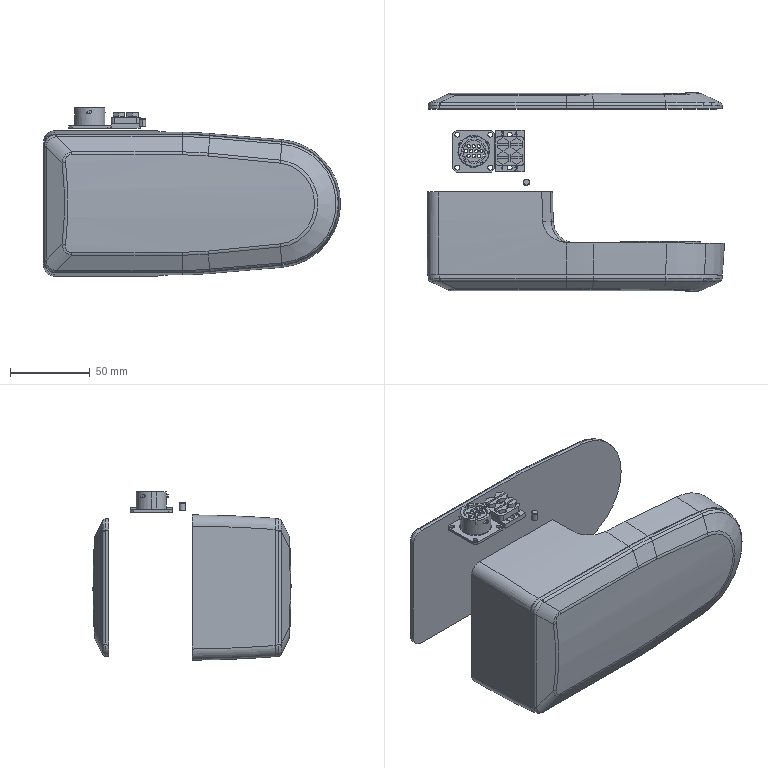Part | STEP file | ASND-0110-IRB120_3-58_IRC5_Link4_rev0-2 | 10 solids | 432 faces | box 186.08 x 124 x 105.45 mm | volume 774376 mm3 | plane 197 | cylinder 130 | spline 55 | cone 33 | torus 13 | other 4 | commonest cylinder face diameters 2 x20 2.2 x20 4 x16 3.1 x8 15.3 x6 17.4 x6